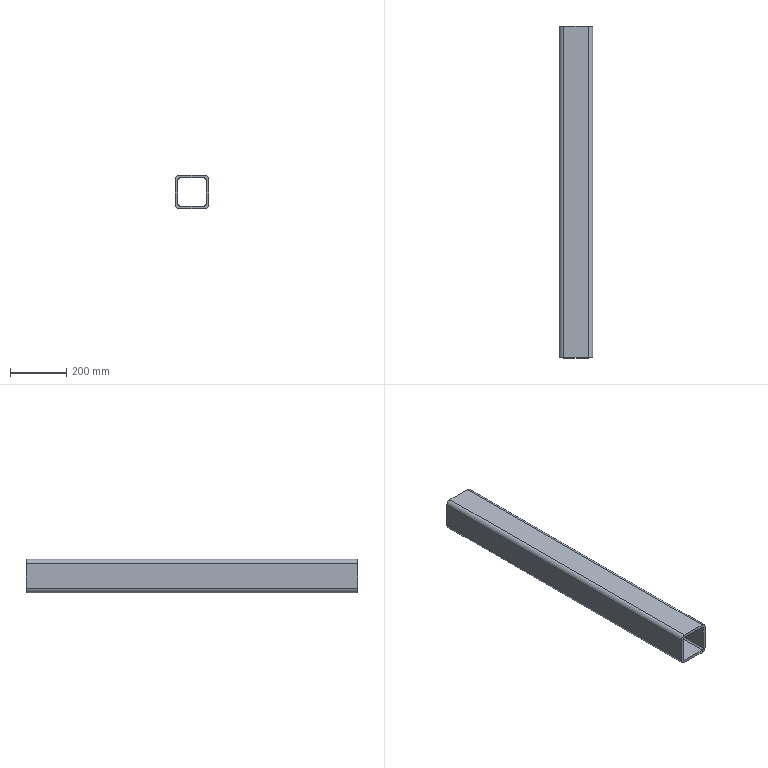Part | SolidWorks | features WeldMemberFeat 1, WeldmentFeature 1 | 1 solid | 18 faces | box 120 x 1185 x 120 mm | volume 4990213 mm3 | plane 10 | cylinder 8 | commonest cylinder face diameters 12 x4 32 x4
STEP:
#1=CARTESIAN_POINT('',(-60.,0.,44.));
#2=VERTEX_POINT('',#1);
#3=CARTESIAN_POINT('',(-44.,0.,60.));
#4=VERTEX_POINT('',#3);
#5=CARTESIAN_POINT('',(-44.,0.,44.));
#6=DIRECTION('',(0.,1.,0.));
#7=DIRECTION('',(0.,0.,1.));
#8=AXIS2_PLACEMENT_3D('',#5,#6,#7);
#9=CIRCLE('',#8,16.);
#10=EDGE_CURVE('',#2,#4,#9,.T.);
#11=ORIENTED_EDGE('',*,*,#10,.T.);
#12=CARTESIAN_POINT('',(-44.,1185.,60.));
#13=VERTEX_POINT('',#12);
#14=CARTESIAN_POINT('',(-44.,1185.,60.));
#15=DIRECTION('',(0.,-1.,0.));
#16=VECTOR('',#15,1000.);
#17=LINE('',#14,#16);
#18=EDGE_CURVE('',#13,#4,#17,.T.);
#19=ORIENTED_EDGE('',*,*,#18,.F.);
#20=CARTESIAN_POINT('',(-60.,1185.,44.));
#21=VERTEX_POINT('',#20);
#22=CARTESIAN_POINT('',(-44.,1185.,44.));
#23=DIRECTION('',(0.,1.,0.));
#24=DIRECTION('',(0.,0.,1.));
#25=AXIS2_PLACEMENT_3D('',#22,#23,#24);
#26=CIRCLE('',#25,16.);
#27=EDGE_CURVE('',#21,#13,#26,.T.);
#28=ORIENTED_EDGE('',*,*,#27,.F.);
#29=CARTESIAN_POINT('',(-60.,1185.,44.));
#30=DIRECTION('',(0.,-1.,0.));
#31=VECTOR('',#30,1000.);
#32=LINE('',#29,#31);
#33=EDGE_CURVE('',#21,#2,#32,.T.);
#34=ORIENTED_EDGE('',*,*,#33,.T.);
#35=EDGE_LOOP('',(#11,#19,#28,#34));
#36=FACE_OUTER_BOUND('',#35,.T.);
#37=CARTESIAN_POINT('',(-44.,1185.,44.));
#38=DIRECTION('',(0.,-1.,0.));
#39=DIRECTION('',(0.,0.,-1.));
#40=AXIS2_PLACEMENT_3D('',#37,#38,#39);
#41=CYLINDRICAL_SURFACE('',#40,16.);
#42=ADVANCED_FACE('',(#36),#41,.T.);
#43=CARTESIAN_POINT('',(44.,0.,60.));
#44=VERTEX_POINT('',#43);
#45=CARTESIAN_POINT('',(-44.,0.,60.));
#46=DIRECTION('',(1.,0.,0.));
#47=VECTOR('',#46,1000.);
#48=LINE('',#45,#47);
#49=EDGE_CURVE('',#4,#44,#48,.T.);
#50=ORIENTED_EDGE('',*,*,#49,.T.);
#51=CARTESIAN_POINT('',(44.,1185.,60.));
#52=VERTEX_POINT('',#51);
#53=CARTESIAN_POINT('',(44.,1185.,60.));
#54=DIRECTION('',(0.,-1.,0.));
#55=VECTOR('',#54,1000.);
#56=LINE('',#53,#55);
#57=EDGE_CURVE('',#52,#44,#56,.T.);
#58=ORIENTED_EDGE('',*,*,#57,.F.);
#59=CARTESIAN_POINT('',(-44.,1185.,60.));
#60=DIRECTION('',(1.,0.,0.));
#61=VECTOR('',#60,1000.);
#62=LINE('',#59,#61);
#63=EDGE_CURVE('',#13,#52,#62,.T.);
#64=ORIENTED_EDGE('',*,*,#63,.F.);
#65=ORIENTED_EDGE('',*,*,#18,.T.);
#66=EDGE_LOOP('',(#50,#58,#64,#65));
#67=FACE_OUTER_BOUND('',#66,.T.);
#68=CARTESIAN_POINT('',(-44.,1185.,60.));
#69=DIRECTION('',(0.,0.,-1.));
#70=DIRECTION('',(-1.,0.,0.));
#71=AXIS2_PLACEMENT_3D('',#68,#69,#70);
#72=PLANE('',#71);
#73=ADVANCED_FACE('',(#67),#72,.F.);
#74=CARTESIAN_POINT('',(60.,0.,44.));
#75=VERTEX_POINT('',#74);
#76=CARTESIAN_POINT('',(44.,0.,44.));
#77=DIRECTION('',(0.,1.,0.));
#78=DIRECTION('',(0.,0.,1.));
#79=AXIS2_PLACEMENT_3D('',#76,#77,#78);
#80=CIRCLE('',#79,16.);
#81=EDGE_CURVE('',#44,#75,#80,.T.);
#82=ORIENTED_EDGE('',*,*,#81,.T.);
#83=CARTESIAN_POINT('',(60.,1185.,44.));
#84=VERTEX_POINT('',#83);
#85=CARTESIAN_POINT('',(60.,1185.,44.));
#86=DIRECTION('',(0.,-1.,0.));
#87=VECTOR('',#86,1000.);
#88=LINE('',#85,#87);
#89=EDGE_CURVE('',#84,#75,#88,.T.);
#90=ORIENTED_EDGE('',*,*,#89,.F.);
#91=CARTESIAN_POINT('',(44.,1185.,44.));
#92=DIRECTION('',(0.,1.,0.));
#93=DIRECTION('',(0.,0.,1.));
#94=AXIS2_PLACEMENT_3D('',#91,#92,#93);
#95=CIRCLE('',#94,16.);
#96=EDGE_CURVE('',#52,#84,#95,.T.);
#97=ORIENTED_EDGE('',*,*,#96,.F.);
#98=ORIENTED_EDGE('',*,*,#57,.T.);
#99=EDGE_LOOP('',(#82,#90,#97,#98));
#100=FACE_OUTER_BOUND('',#99,.T.);
#101=CARTESIAN_POINT('',(44.,1185.,44.));
#102=DIRECTION('',(0.,-1.,0.));
#103=DIRECTION('',(0.,0.,-1.));
#104=AXIS2_PLACEMENT_3D('',#101,#102,#103);
#105=CYLINDRICAL_SURFACE('',#104,16.);
#106=ADVANCED_FACE('',(#100),#105,.T.);
#107=CARTESIAN_POINT('',(60.,0.,-44.));
#108=VERTEX_POINT('',#107);
#109=CARTESIAN_POINT('',(60.,0.,-44.));
#110=DIRECTION('',(0.,0.,-1.));
#111=VECTOR('',#110,1000.);
#112=LINE('',#109,#111);
#113=EDGE_CURVE('',#75,#108,#112,.T.);
#114=ORIENTED_EDGE('',*,*,#113,.T.);
#115=CARTESIAN_POINT('',(60.,1185.,-44.));
#116=VERTEX_POINT('',#115);
#117=CARTESIAN_POINT('',(60.,1185.,-44.));
#118=DIRECTION('',(0.,-1.,0.));
#119=VECTOR('',#118,1000.);
#120=LINE('',#117,#119);
#121=EDGE_CURVE('',#116,#108,#120,.T.);
#122=ORIENTED_EDGE('',*,*,#121,.F.);
#123=CARTESIAN_POINT('',(60.,1185.,-44.));
#124=DIRECTION('',(0.,0.,-1.));
#125=VECTOR('',#124,1000.);
#126=LINE('',#123,#125);
#127=EDGE_CURVE('',#84,#116,#126,.T.);
#128=ORIENTED_EDGE('',*,*,#127,.F.);
#129=ORIENTED_EDGE('',*,*,#89,.T.);
#130=EDGE_LOOP('',(#114,#122,#128,#129));
#131=FACE_OUTER_BOUND('',#130,.T.);
#132=CARTESIAN_POINT('',(60.,1185.,-44.));
#133=DIRECTION('',(-1.,0.,0.));
#134=DIRECTION('',(0.,0.,1.));
#135=AXIS2_PLACEMENT_3D('',#132,#133,#134);
#136=PLANE('',#135);
#137=ADVANCED_FACE('',(#131),#136,.F.);
#138=CARTESIAN_POINT('',(44.,0.,-60.));
#139=VERTEX_POINT('',#138);
#140=CARTESIAN_POINT('',(44.,0.,-44.));
#141=DIRECTION('',(0.,1.,0.));
#142=DIRECTION('',(0.,0.,1.));
#143=AXIS2_PLACEMENT_3D('',#140,#141,#142);
#144=CIRCLE('',#143,16.);
#145=EDGE_CURVE('',#108,#139,#144,.T.);
#146=ORIENTED_EDGE('',*,*,#145,.T.);
#147=CARTESIAN_POINT('',(44.,1185.,-60.));
#148=VERTEX_POINT('',#147);
#149=CARTESIAN_POINT('',(44.,1185.,-60.));
#150=DIRECTION('',(0.,-1.,0.));
#151=VECTOR('',#150,1000.);
#152=LINE('',#149,#151);
#153=EDGE_CURVE('',#148,#139,#152,.T.);
#154=ORIENTED_EDGE('',*,*,#153,.F.);
#155=CARTESIAN_POINT('',(44.,1185.,-44.));
#156=DIRECTION('',(0.,1.,0.));
#157=DIRECTION('',(0.,0.,1.));
#158=AXIS2_PLACEMENT_3D('',#155,#156,#157);
#159=CIRCLE('',#158,16.);
#160=EDGE_CURVE('',#116,#148,#159,.T.);
#161=ORIENTED_EDGE('',*,*,#160,.F.);
#162=ORIENTED_EDGE('',*,*,#121,.T.);
#163=EDGE_LOOP('',(#146,#154,#161,#162));
#164=FACE_OUTER_BOUND('',#163,.T.);
#165=CARTESIAN_POINT('',(44.,1185.,-44.));
#166=DIRECTION('',(0.,-1.,0.));
#167=DIRECTION('',(0.,0.,-1.));
#168=AXIS2_PLACEMENT_3D('',#165,#166,#167);
#169=CYLINDRICAL_SURFACE('',#168,16.);
#170=ADVANCED_FACE('',(#164),#169,.T.);
#171=CARTESIAN_POINT('',(-44.,0.,-60.));
#172=VERTEX_POINT('',#171);
#173=CARTESIAN_POINT('',(44.,0.,-60.));
#174=DIRECTION('',(-1.,0.,0.));
#175=VECTOR('',#174,1000.);
#176=LINE('',#173,#175);
#177=EDGE_CURVE('',#139,#172,#176,.T.);
#178=ORIENTED_EDGE('',*,*,#177,.T.);
#179=CARTESIAN_POINT('',(-44.,1185.,-60.));
#180=VERTEX_POINT('',#179);
#181=CARTESIAN_POINT('',(-44.,1185.,-60.));
#182=DIRECTION('',(0.,-1.,0.));
#183=VECTOR('',#182,1000.);
#184=LINE('',#181,#183);
#185=EDGE_CURVE('',#180,#172,#184,.T.);
#186=ORIENTED_EDGE('',*,*,#185,.F.);
#187=CARTESIAN_POINT('',(44.,1185.,-60.));
#188=DIRECTION('',(-1.,0.,0.));
#189=VECTOR('',#188,1000.);
#190=LINE('',#187,#189);
#191=EDGE_CURVE('',#148,#180,#190,.T.);
#192=ORIENTED_EDGE('',*,*,#191,.F.);
#193=ORIENTED_EDGE('',*,*,#153,.T.);
#194=EDGE_LOOP('',(#178,#186,#192,#193));
#195=FACE_OUTER_BOUND('',#194,.T.);
#196=CARTESIAN_POINT('',(44.,1185.,-60.));
#197=DIRECTION('',(0.,0.,1.));
#198=DIRECTION('',(1.,0.,0.));
#199=AXIS2_PLACEMENT_3D('',#196,#197,#198);
#200=PLANE('',#199);
#201=ADVANCED_FACE('',(#195),#200,.F.);
#202=CARTESIAN_POINT('',(-60.,0.,-44.));
#203=VERTEX_POINT('',#202);
#204=CARTESIAN_POINT('',(-44.,0.,-44.));
#205=DIRECTION('',(0.,1.,0.));
#206=DIRECTION('',(0.,0.,1.));
#207=AXIS2_PLACEMENT_3D('',#204,#205,#206);
#208=CIRCLE('',#207,16.);
#209=EDGE_CURVE('',#172,#203,#208,.T.);
#210=ORIENTED_EDGE('',*,*,#209,.T.);
#211=CARTESIAN_POINT('',(-60.,1185.,-44.));
#212=VERTEX_POINT('',#211);
#213=CARTESIAN_POINT('',(-60.,1185.,-44.));
#214=DIRECTION('',(0.,-1.,0.));
#215=VECTOR('',#214,1000.);
#216=LINE('',#213,#215);
#217=EDGE_CURVE('',#212,#203,#216,.T.);
#218=ORIENTED_EDGE('',*,*,#217,.F.);
#219=CARTESIAN_POINT('',(-44.,1185.,-44.));
#220=DIRECTION('',(0.,1.,0.));
#221=DIRECTION('',(0.,0.,1.));
#222=AXIS2_PLACEMENT_3D('',#219,#220,#221);
#223=CIRCLE('',#222,16.);
#224=EDGE_CURVE('',#180,#212,#223,.T.);
#225=ORIENTED_EDGE('',*,*,#224,.F.);
#226=ORIENTED_EDGE('',*,*,#185,.T.);
#227=EDGE_LOOP('',(#210,#218,#225,#226));
#228=FACE_OUTER_BOUND('',#227,.T.);
#229=CARTESIAN_POINT('',(-44.,1185.,-44.));
#230=DIRECTION('',(0.,-1.,0.));
#231=DIRECTION('',(0.,0.,-1.));
#232=AXIS2_PLACEMENT_3D('',#229,#230,#231);
#233=CYLINDRICAL_SURFACE('',#232,16.);
#234=ADVANCED_FACE('',(#228),#233,.T.);
#235=CARTESIAN_POINT('',(44.,0.,50.));
#236=VERTEX_POINT('',#235);
#237=CARTESIAN_POINT('',(50.,0.,44.));
#238=VERTEX_POINT('',#237);
#239=CARTESIAN_POINT('',(44.,0.,44.));
#240=DIRECTION('',(0.,1.,0.));
#241=DIRECTION('',(0.,0.,1.));
#242=AXIS2_PLACEMENT_3D('',#239,#240,#241);
#243=CIRCLE('',#242,6.);
#244=EDGE_CURVE('',#236,#238,#243,.T.);
#245=ORIENTED_EDGE('',*,*,#244,.F.);
#246=CARTESIAN_POINT('',(44.,1185.,50.));
#247=VERTEX_POINT('',#246);
#248=CARTESIAN_POINT('',(44.,1185.,50.));
#249=DIRECTION('',(0.,-1.,0.));
#250=VECTOR('',#249,1000.);
#251=LINE('',#248,#250);
#252=EDGE_CURVE('',#247,#236,#251,.T.);
#253=ORIENTED_EDGE('',*,*,#252,.F.);
#254=CARTESIAN_POINT('',(50.,1185.,44.));
#255=VERTEX_POINT('',#254);
#256=CARTESIAN_POINT('',(44.,1185.,44.));
#257=DIRECTION('',(0.,1.,0.));
#258=DIRECTION('',(0.,0.,1.));
#259=AXIS2_PLACEMENT_3D('',#256,#257,#258);
#260=CIRCLE('',#259,6.);
#261=EDGE_CURVE('',#247,#255,#260,.T.);
#262=ORIENTED_EDGE('',*,*,#261,.T.);
#263=CARTESIAN_POINT('',(50.,1185.,44.));
#264=DIRECTION('',(0.,-1.,0.));
#265=VECTOR('',#264,1000.);
#266=LINE('',#263,#265);
#267=EDGE_CURVE('',#255,#238,#266,.T.);
#268=ORIENTED_EDGE('',*,*,#267,.T.);
#269=EDGE_LOOP('',(#245,#253,#262,#268));
#270=FACE_OUTER_BOUND('',#269,.T.);
#271=CARTESIAN_POINT('',(44.,1185.,44.));
#272=DIRECTION('',(0.,-1.,0.));
#273=DIRECTION('',(0.,0.,-1.));
#274=AXIS2_PLACEMENT_3D('',#271,#272,#273);
#275=CYLINDRICAL_SURFACE('',#274,6.);
#276=ADVANCED_FACE('',(#270),#275,.F.);
#277=CARTESIAN_POINT('',(-44.,0.,50.));
#278=VERTEX_POINT('',#277);
#279=CARTESIAN_POINT('',(-44.,0.,50.));
#280=DIRECTION('',(1.,0.,0.));
#281=VECTOR('',#280,1000.);
#282=LINE('',#279,#281);
#283=EDGE_CURVE('',#278,#236,#282,.T.);
#284=ORIENTED_EDGE('',*,*,#283,.F.);
#285=CARTESIAN_POINT('',(-44.,1185.,50.));
#286=VERTEX_POINT('',#285);
#287=CARTESIAN_POINT('',(-44.,1185.,50.));
#288=DIRECTION('',(0.,-1.,0.));
#289=VECTOR('',#288,1000.);
#290=LINE('',#287,#289);
#291=EDGE_CURVE('',#286,#278,#290,.T.);
#292=ORIENTED_EDGE('',*,*,#291,.F.);
#293=CARTESIAN_POINT('',(-44.,1185.,50.));
#294=DIRECTION('',(1.,0.,0.));
#295=VECTOR('',#294,1000.);
#296=LINE('',#293,#295);
#297=EDGE_CURVE('',#286,#247,#296,.T.);
#298=ORIENTED_EDGE('',*,*,#297,.T.);
#299=ORIENTED_EDGE('',*,*,#252,.T.);
#300=EDGE_LOOP('',(#284,#292,#298,#299));
#301=FACE_OUTER_BOUND('',#300,.T.);
#302=CARTESIAN_POINT('',(-44.,1185.,50.));
#303=DIRECTION('',(0.,0.,-1.));
#304=DIRECTION('',(-1.,0.,0.));
#305=AXIS2_PLACEMENT_3D('',#302,#303,#304);
#306=PLANE('',#305);
#307=ADVANCED_FACE('',(#301),#306,.T.);
#308=CARTESIAN_POINT('',(-50.,0.,44.));
#309=VERTEX_POINT('',#308);
#310=CARTESIAN_POINT('',(-44.,0.,44.));
#311=DIRECTION('',(0.,1.,0.));
#312=DIRECTION('',(0.,0.,1.));
#313=AXIS2_PLACEMENT_3D('',#310,#311,#312);
#314=CIRCLE('',#313,6.);
#315=EDGE_CURVE('',#309,#278,#314,.T.);
#316=ORIENTED_EDGE('',*,*,#315,.F.);
#317=CARTESIAN_POINT('',(-50.,1185.,44.));
#318=VERTEX_POINT('',#317);
#319=CARTESIAN_POINT('',(-50.,1185.,44.));
#320=DIRECTION('',(0.,-1.,0.));
#321=VECTOR('',#320,1000.);
#322=LINE('',#319,#321);
#323=EDGE_CURVE('',#318,#309,#322,.T.);
#324=ORIENTED_EDGE('',*,*,#323,.F.);
#325=CARTESIAN_POINT('',(-44.,1185.,44.));
#326=DIRECTION('',(0.,1.,0.));
#327=DIRECTION('',(0.,0.,1.));
#328=AXIS2_PLACEMENT_3D('',#325,#326,#327);
#329=CIRCLE('',#328,6.);
#330=EDGE_CURVE('',#318,#286,#329,.T.);
#331=ORIENTED_EDGE('',*,*,#330,.T.);
#332=ORIENTED_EDGE('',*,*,#291,.T.);
#333=EDGE_LOOP('',(#316,#324,#331,#332));
#334=FACE_OUTER_BOUND('',#333,.T.);
#335=CARTESIAN_POINT('',(-44.,1185.,44.));
#336=DIRECTION('',(0.,-1.,0.));
#337=DIRECTION('',(0.,0.,-1.));
#338=AXIS2_PLACEMENT_3D('',#335,#336,#337);
#339=CYLINDRICAL_SURFACE('',#338,6.);
#340=ADVANCED_FACE('',(#334),#339,.F.);
#341=CARTESIAN_POINT('',(-50.,0.,-44.));
#342=VERTEX_POINT('',#341);
#343=CARTESIAN_POINT('',(-50.,0.,44.));
#344=DIRECTION('',(0.,0.,1.));
#345=VECTOR('',#344,1000.);
#346=LINE('',#343,#345);
#347=EDGE_CURVE('',#342,#309,#346,.T.);
#348=ORIENTED_EDGE('',*,*,#347,.F.);
#349=CARTESIAN_POINT('',(-50.,1185.,-44.));
#350=VERTEX_POINT('',#349);
#351=CARTESIAN_POINT('',(-50.,1185.,-44.));
#352=DIRECTION('',(0.,-1.,0.));
#353=VECTOR('',#352,1000.);
#354=LINE('',#351,#353);
#355=EDGE_CURVE('',#350,#342,#354,.T.);
#356=ORIENTED_EDGE('',*,*,#355,.F.);
#357=CARTESIAN_POINT('',(-50.,1185.,44.));
#358=DIRECTION('',(0.,0.,1.));
#359=VECTOR('',#358,1000.);
#360=LINE('',#357,#359);
#361=EDGE_CURVE('',#350,#318,#360,.T.);
#362=ORIENTED_EDGE('',*,*,#361,.T.);
#363=ORIENTED_EDGE('',*,*,#323,.T.);
#364=EDGE_LOOP('',(#348,#356,#362,#363));
#365=FACE_OUTER_BOUND('',#364,.T.);
#366=CARTESIAN_POINT('',(-50.,1185.,44.));
#367=DIRECTION('',(1.,0.,0.));
#368=DIRECTION('',(0.,0.,-1.));
#369=AXIS2_PLACEMENT_3D('',#366,#367,#368);
#370=PLANE('',#369);
#371=ADVANCED_FACE('',(#365),#370,.T.);
#372=CARTESIAN_POINT('',(-44.,0.,-50.));
#373=VERTEX_POINT('',#372);
#374=CARTESIAN_POINT('',(-44.,0.,-44.));
#375=DIRECTION('',(0.,1.,0.));
#376=DIRECTION('',(0.,0.,1.));
#377=AXIS2_PLACEMENT_3D('',#374,#375,#376);
#378=CIRCLE('',#377,6.);
#379=EDGE_CURVE('',#373,#342,#378,.T.);
#380=ORIENTED_EDGE('',*,*,#379,.F.);
#381=CARTESIAN_POINT('',(-44.,1185.,-50.));
#382=VERTEX_POINT('',#381);
#383=CARTESIAN_POINT('',(-44.,1185.,-50.));
#384=DIRECTION('',(0.,-1.,0.));
#385=VECTOR('',#384,1000.);
#386=LINE('',#383,#385);
#387=EDGE_CURVE('',#382,#373,#386,.T.);
#388=ORIENTED_EDGE('',*,*,#387,.F.);
#389=CARTESIAN_POINT('',(-44.,1185.,-44.));
#390=DIRECTION('',(0.,1.,0.));
#391=DIRECTION('',(0.,0.,1.));
#392=AXIS2_PLACEMENT_3D('',#389,#390,#391);
#393=CIRCLE('',#392,6.);
#394=EDGE_CURVE('',#382,#350,#393,.T.);
#395=ORIENTED_EDGE('',*,*,#394,.T.);
#396=ORIENTED_EDGE('',*,*,#355,.T.);
#397=EDGE_LOOP('',(#380,#388,#395,#396));
#398=FACE_OUTER_BOUND('',#397,.T.);
#399=CARTESIAN_POINT('',(-44.,1185.,-44.));
#400=DIRECTION('',(0.,-1.,0.));
#401=DIRECTION('',(0.,0.,-1.));
#402=AXIS2_PLACEMENT_3D('',#399,#400,#401);
#403=CYLINDRICAL_SURFACE('',#402,6.);
#404=ADVANCED_FACE('',(#398),#403,.F.);
#405=CARTESIAN_POINT('',(44.,0.,-50.));
#406=VERTEX_POINT('',#405);
#407=CARTESIAN_POINT('',(44.,0.,-50.));
#408=DIRECTION('',(-1.,0.,0.));
#409=VECTOR('',#408,1000.);
#410=LINE('',#407,#409);
#411=EDGE_CURVE('',#406,#373,#410,.T.);
#412=ORIENTED_EDGE('',*,*,#411,.F.);
#413=CARTESIAN_POINT('',(44.,1185.,-50.));
#414=VERTEX_POINT('',#413);
#415=CARTESIAN_POINT('',(44.,1185.,-50.));
#416=DIRECTION('',(0.,-1.,0.));
#417=VECTOR('',#416,1000.);
#418=LINE('',#415,#417);
#419=EDGE_CURVE('',#414,#406,#418,.T.);
#420=ORIENTED_EDGE('',*,*,#419,.F.);
#421=CARTESIAN_POINT('',(44.,1185.,-50.));
#422=DIRECTION('',(-1.,0.,0.));
#423=VECTOR('',#422,1000.);
#424=LINE('',#421,#423);
#425=EDGE_CURVE('',#414,#382,#424,.T.);
#426=ORIENTED_EDGE('',*,*,#425,.T.);
#427=ORIENTED_EDGE('',*,*,#387,.T.);
#428=EDGE_LOOP('',(#412,#420,#426,#427));
#429=FACE_OUTER_BOUND('',#428,.T.);
#430=CARTESIAN_POINT('',(44.,1185.,-50.));
#431=DIRECTION('',(0.,0.,1.));
#432=DIRECTION('',(1.,0.,0.));
#433=AXIS2_PLACEMENT_3D('',#430,#431,#432);
#434=PLANE('',#433);
#435=ADVANCED_FACE('',(#429),#434,.T.);
#436=CARTESIAN_POINT('',(50.,0.,-44.));
#437=VERTEX_POINT('',#436);
#438=CARTESIAN_POINT('',(44.,0.,-44.));
#439=DIRECTION('',(0.,1.,0.));
#440=DIRECTION('',(0.,0.,1.));
#441=AXIS2_PLACEMENT_3D('',#438,#439,#440);
#442=CIRCLE('',#441,6.);
#443=EDGE_CURVE('',#437,#406,#442,.T.);
#444=ORIENTED_EDGE('',*,*,#443,.F.);
#445=CARTESIAN_POINT('',(50.,1185.,-44.));
#446=VERTEX_POINT('',#445);
#447=CARTESIAN_POINT('',(50.,1185.,-44.));
#448=DIRECTION('',(0.,-1.,0.));
#449=VECTOR('',#448,1000.);
#450=LINE('',#447,#449);
#451=EDGE_CURVE('',#446,#437,#450,.T.);
#452=ORIENTED_EDGE('',*,*,#451,.F.);
#453=CARTESIAN_POINT('',(44.,1185.,-44.));
#454=DIRECTION('',(0.,1.,0.));
#455=DIRECTION('',(0.,0.,1.));
#456=AXIS2_PLACEMENT_3D('',#453,#454,#455);
#457=CIRCLE('',#456,6.);
#458=EDGE_CURVE('',#446,#414,#457,.T.);
#459=ORIENTED_EDGE('',*,*,#458,.T.);
#460=ORIENTED_EDGE('',*,*,#419,.T.);
#461=EDGE_LOOP('',(#444,#452,#459,#460));
#462=FACE_OUTER_BOUND('',#461,.T.);
#463=CARTESIAN_POINT('',(44.,1185.,-44.));
#464=DIRECTION('',(0.,-1.,0.));
#465=DIRECTION('',(0.,0.,-1.));
#466=AXIS2_PLACEMENT_3D('',#463,#464,#465);
#467=CYLINDRICAL_SURFACE('',#466,6.);
#468=ADVANCED_FACE('',(#462),#467,.F.);
#469=CARTESIAN_POINT('',(50.,0.,-44.));
#470=DIRECTION('',(0.,0.,-1.));
#471=VECTOR('',#470,1000.);
#472=LINE('',#469,#471);
#473=EDGE_CURVE('',#238,#437,#472,.T.);
#474=ORIENTED_EDGE('',*,*,#473,.F.);
#475=ORIENTED_EDGE('',*,*,#267,.F.);
#476=CARTESIAN_POINT('',(50.,1185.,-44.));
#477=DIRECTION('',(0.,0.,-1.));
#478=VECTOR('',#477,1000.);
#479=LINE('',#476,#478);
#480=EDGE_CURVE('',#255,#446,#479,.T.);
#481=ORIENTED_EDGE('',*,*,#480,.T.);
#482=ORIENTED_EDGE('',*,*,#451,.T.);
#483=EDGE_LOOP('',(#474,#475,#481,#482));
#484=FACE_OUTER_BOUND('',#483,.T.);
#485=CARTESIAN_POINT('',(50.,1185.,-44.));
#486=DIRECTION('',(-1.,0.,0.));
#487=DIRECTION('',(0.,0.,1.));
#488=AXIS2_PLACEMENT_3D('',#485,#486,#487);
#489=PLANE('',#488);
#490=ADVANCED_FACE('',(#484),#489,.T.);
#491=CARTESIAN_POINT('',(-60.,0.,44.));
#492=DIRECTION('',(0.,0.,1.));
#493=VECTOR('',#492,1000.);
#494=LINE('',#491,#493);
#495=EDGE_CURVE('',#203,#2,#494,.T.);
#496=ORIENTED_EDGE('',*,*,#495,.T.);
#497=ORIENTED_EDGE('',*,*,#33,.F.);
#498=CARTESIAN_POINT('',(-60.,1185.,44.));
#499=DIRECTION('',(0.,0.,1.));
#500=VECTOR('',#499,1000.);
#501=LINE('',#498,#500);
#502=EDGE_CURVE('',#212,#21,#501,.T.);
#503=ORIENTED_EDGE('',*,*,#502,.F.);
#504=ORIENTED_EDGE('',*,*,#217,.T.);
#505=EDGE_LOOP('',(#496,#497,#503,#504));
#506=FACE_OUTER_BOUND('',#505,.T.);
#507=CARTESIAN_POINT('',(-60.,1185.,44.));
#508=DIRECTION('',(1.,0.,0.));
#509=DIRECTION('',(0.,0.,-1.));
#510=AXIS2_PLACEMENT_3D('',#507,#508,#509);
#511=PLANE('',#510);
#512=ADVANCED_FACE('',(#506),#511,.F.);
#513=ORIENTED_EDGE('',*,*,#261,.F.);
#514=ORIENTED_EDGE('',*,*,#297,.F.);
#515=ORIENTED_EDGE('',*,*,#330,.F.);
#516=ORIENTED_EDGE('',*,*,#361,.F.);
#517=ORIENTED_EDGE('',*,*,#394,.F.);
#518=ORIENTED_EDGE('',*,*,#425,.F.);
#519=ORIENTED_EDGE('',*,*,#458,.F.);
#520=ORIENTED_EDGE('',*,*,#480,.F.);
#521=EDGE_LOOP('',(#513,#514,#515,#516,#517,#518,#519,#520));
#522=FACE_BOUND('',#521,.T.);
#523=ORIENTED_EDGE('',*,*,#27,.T.);
#524=ORIENTED_EDGE('',*,*,#63,.T.);
#525=ORIENTED_EDGE('',*,*,#96,.T.);
#526=ORIENTED_EDGE('',*,*,#127,.T.);
#527=ORIENTED_EDGE('',*,*,#160,.T.);
#528=ORIENTED_EDGE('',*,*,#191,.T.);
#529=ORIENTED_EDGE('',*,*,#224,.T.);
#530=ORIENTED_EDGE('',*,*,#502,.T.);
#531=EDGE_LOOP('',(#523,#524,#525,#526,#527,#528,#529,#530));
#532=FACE_OUTER_BOUND('',#531,.T.);
#533=CARTESIAN_POINT('',(-44.,1185.,44.));
#534=DIRECTION('',(0.,1.,0.));
#535=DIRECTION('',(0.,0.,1.));
#536=AXIS2_PLACEMENT_3D('',#533,#534,#535);
#537=PLANE('',#536);
#538=ADVANCED_FACE('',(#522,#532),#537,.T.);
#539=ORIENTED_EDGE('',*,*,#244,.T.);
#540=ORIENTED_EDGE('',*,*,#473,.T.);
#541=ORIENTED_EDGE('',*,*,#443,.T.);
#542=ORIENTED_EDGE('',*,*,#411,.T.);
#543=ORIENTED_EDGE('',*,*,#379,.T.);
#544=ORIENTED_EDGE('',*,*,#347,.T.);
#545=ORIENTED_EDGE('',*,*,#315,.T.);
#546=ORIENTED_EDGE('',*,*,#283,.T.);
#547=EDGE_LOOP('',(#539,#540,#541,#542,#543,#544,#545,#546));
#548=FACE_BOUND('',#547,.T.);
#549=ORIENTED_EDGE('',*,*,#10,.F.);
#550=ORIENTED_EDGE('',*,*,#495,.F.);
#551=ORIENTED_EDGE('',*,*,#209,.F.);
#552=ORIENTED_EDGE('',*,*,#177,.F.);
#553=ORIENTED_EDGE('',*,*,#145,.F.);
#554=ORIENTED_EDGE('',*,*,#113,.F.);
#555=ORIENTED_EDGE('',*,*,#81,.F.);
#556=ORIENTED_EDGE('',*,*,#49,.F.);
#557=EDGE_LOOP('',(#549,#550,#551,#552,#553,#554,#555,#556));
#558=FACE_OUTER_BOUND('',#557,.T.);
#559=CARTESIAN_POINT('',(-44.,0.,44.));
#560=DIRECTION('',(0.,1.,0.));
#561=DIRECTION('',(0.,0.,1.));
#562=AXIS2_PLACEMENT_3D('',#559,#560,#561);
#563=PLANE('',#562);
#564=ADVANCED_FACE('',(#548,#558),#563,.F.);
#565=CLOSED_SHELL('',(#42,#73,#106,#137,#170,#201,#234,#276,#307,#340,#371,#404,#435,#468,#490,#512,#538,#564));
#566=MANIFOLD_SOLID_BREP('',#565);
#567=CARTESIAN_POINT('',(0.,0.,0.));
#568=DIRECTION('',(0.,0.,1.));
#569=DIRECTION('',(1.,0.,0.));
#570=AXIS2_PLACEMENT_3D('',#567,#568,#569);
#571=(LENGTH_UNIT()NAMED_UNIT(*)SI_UNIT(.MILLI.,.METRE.));
#572=UNCERTAINTY_MEASURE_WITH_UNIT(LENGTH_MEASURE(0.00001),#571,'','');
#573=(NAMED_UNIT(*)PLANE_ANGLE_UNIT()SI_UNIT($,.RADIAN.));
#574=(NAMED_UNIT(*)SI_UNIT($,.STERADIAN.)SOLID_ANGLE_UNIT());
#575=(GEOMETRIC_REPRESENTATION_CONTEXT(3)GLOBAL_UNCERTAINTY_ASSIGNED_CONTEXT((#572))GLOBAL_UNIT_ASSIGNED_CONTEXT((#571,#573,#574))REPRESENTATION_CONTEXT('',''));
#576=ADVANCED_BREP_SHAPE_REPRESENTATION('',(#566,#570),#575);